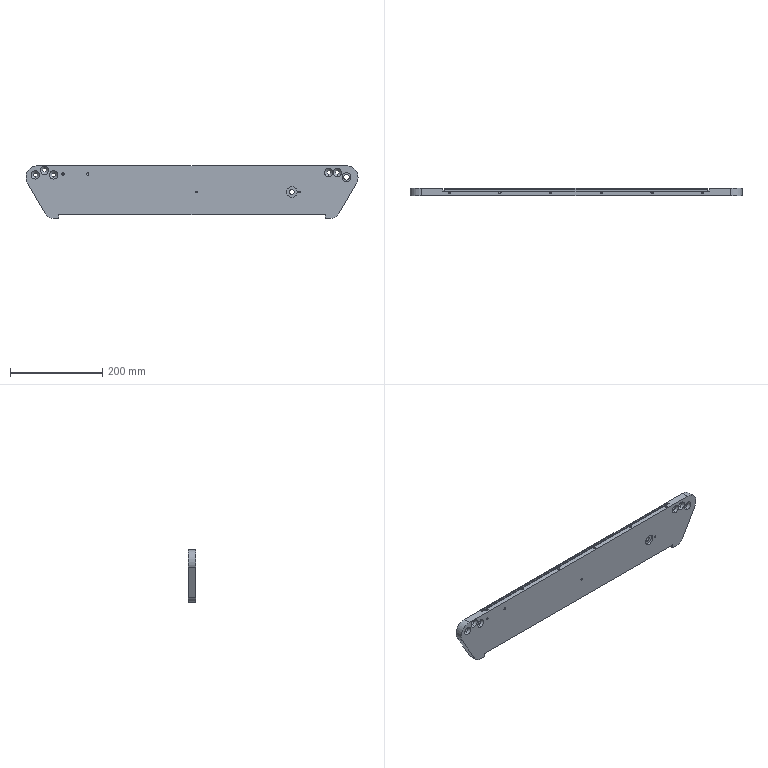Part | SolidWorks | features BaseBody 1 | 1 solid | 122 faces | box 720.1 x 16 x 114 mm | volume 1136036 mm3 | cylinder 54 | cone 42 | plane 26 | commonest cylinder face diameters 5 x28 8.4 x10 4.2 x4 10.2 x2 12.06 x2 19 x2